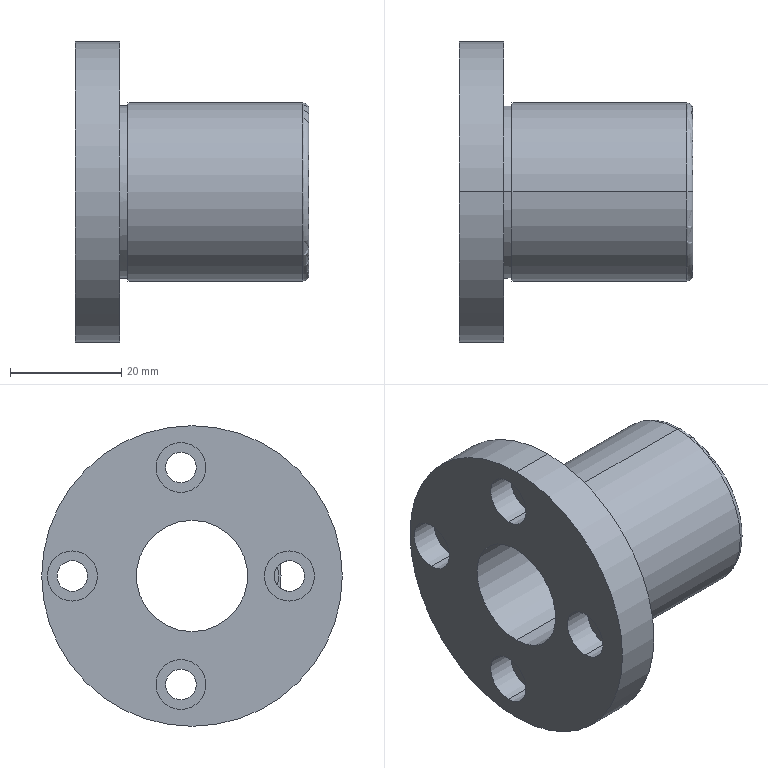Part | STEP file | LHFR20_LHTR20 | 1 solid | 35 faces | box 42 x 54 x 54 mm | volume 30800 mm3 | cylinder 24 | plane 9 | torus 2 | commonest cylinder face diameters 5.5 x8 9 x8 20 x2 31 x2 32 x2 54 x2
STEP:
#1=CARTESIAN_POINT('',(8.,-17.5,-2.75));
#2=VERTEX_POINT('',#1);
#3=CARTESIAN_POINT('',(8.,-17.5,2.75));
#4=VERTEX_POINT('',#3);
#5=CARTESIAN_POINT('',(8.,-17.5,0.));
#6=DIRECTION('',(-1.,0.,0.));
#7=DIRECTION('',(0.,0.,1.));
#8=AXIS2_PLACEMENT_3D('',#5,#6,#7);
#9=CIRCLE('',#8,2.75);
#10=EDGE_CURVE('',#2,#4,#9,.T.);
#11=ORIENTED_EDGE('',*,*,#10,.F.);
#12=CARTESIAN_POINT('',(5.1,-17.5,-2.75));
#13=VERTEX_POINT('',#12);
#14=CARTESIAN_POINT('',(8.,-17.5,-2.75));
#15=DIRECTION('',(-1.,0.,0.));
#16=VECTOR('',#15,1000.);
#17=LINE('',#14,#16);
#18=EDGE_CURVE('',#2,#13,#17,.T.);
#19=ORIENTED_EDGE('',*,*,#18,.T.);
#20=CARTESIAN_POINT('',(5.1,-17.5,2.75));
#21=VERTEX_POINT('',#20);
#22=CARTESIAN_POINT('',(5.1,-17.5,0.));
#23=DIRECTION('',(-1.,0.,0.));
#24=DIRECTION('',(0.,0.,1.));
#25=AXIS2_PLACEMENT_3D('',#22,#23,#24);
#26=CIRCLE('',#25,2.75);
#27=EDGE_CURVE('',#13,#21,#26,.T.);
#28=ORIENTED_EDGE('',*,*,#27,.T.);
#29=CARTESIAN_POINT('',(8.,-17.5,2.75));
#30=DIRECTION('',(-1.,0.,0.));
#31=VECTOR('',#30,1000.);
#32=LINE('',#29,#31);
#33=EDGE_CURVE('',#4,#21,#32,.T.);
#34=ORIENTED_EDGE('',*,*,#33,.F.);
#35=EDGE_LOOP('',(#11,#19,#28,#34));
#36=FACE_OUTER_BOUND('',#35,.T.);
#37=CARTESIAN_POINT('',(8.,-17.5,0.));
#38=DIRECTION('',(-1.,0.,0.));
#39=DIRECTION('',(0.,0.,1.));
#40=AXIS2_PLACEMENT_3D('',#37,#38,#39);
#41=CYLINDRICAL_SURFACE('',#40,2.75);
#42=ADVANCED_FACE('',(#36),#41,.F.);
#43=CARTESIAN_POINT('',(5.1,-17.5,-4.5));
#44=VERTEX_POINT('',#43);
#45=CARTESIAN_POINT('',(5.1,-17.5,4.5));
#46=VERTEX_POINT('',#45);
#47=CARTESIAN_POINT('',(5.1,-17.5,0.));
#48=DIRECTION('',(-1.,0.,0.));
#49=DIRECTION('',(0.,0.,1.));
#50=AXIS2_PLACEMENT_3D('',#47,#48,#49);
#51=CIRCLE('',#50,4.5);
#52=EDGE_CURVE('',#44,#46,#51,.T.);
#53=ORIENTED_EDGE('',*,*,#52,.F.);
#54=CARTESIAN_POINT('',(0.,-17.5,-4.5));
#55=VERTEX_POINT('',#54);
#56=CARTESIAN_POINT('',(8.,-17.5,-4.5));
#57=DIRECTION('',(-1.,0.,0.));
#58=VECTOR('',#57,1000.);
#59=LINE('',#56,#58);
#60=EDGE_CURVE('',#44,#55,#59,.T.);
#61=ORIENTED_EDGE('',*,*,#60,.T.);
#62=CARTESIAN_POINT('',(0.,-17.5,4.5));
#63=VERTEX_POINT('',#62);
#64=CARTESIAN_POINT('',(0.,-17.5,0.));
#65=DIRECTION('',(-1.,0.,0.));
#66=DIRECTION('',(0.,0.,1.));
#67=AXIS2_PLACEMENT_3D('',#64,#65,#66);
#68=CIRCLE('',#67,4.5);
#69=EDGE_CURVE('',#55,#63,#68,.T.);
#70=ORIENTED_EDGE('',*,*,#69,.T.);
#71=CARTESIAN_POINT('',(8.,-17.5,4.5));
#72=DIRECTION('',(-1.,0.,0.));
#73=VECTOR('',#72,1000.);
#74=LINE('',#71,#73);
#75=EDGE_CURVE('',#46,#63,#74,.T.);
#76=ORIENTED_EDGE('',*,*,#75,.F.);
#77=EDGE_LOOP('',(#53,#61,#70,#76));
#78=FACE_OUTER_BOUND('',#77,.T.);
#79=CARTESIAN_POINT('',(8.,-17.5,0.));
#80=DIRECTION('',(-1.,0.,0.));
#81=DIRECTION('',(0.,0.,1.));
#82=AXIS2_PLACEMENT_3D('',#79,#80,#81);
#83=CYLINDRICAL_SURFACE('',#82,4.5);
#84=ADVANCED_FACE('',(#78),#83,.F.);
#85=CARTESIAN_POINT('',(8.,2.,16.75));
#86=VERTEX_POINT('',#85);
#87=CARTESIAN_POINT('',(8.,2.,22.25));
#88=VERTEX_POINT('',#87);
#89=CARTESIAN_POINT('',(8.,2.,19.5));
#90=DIRECTION('',(-1.,0.,0.));
#91=DIRECTION('',(0.,0.,1.));
#92=AXIS2_PLACEMENT_3D('',#89,#90,#91);
#93=CIRCLE('',#92,2.75);
#94=EDGE_CURVE('',#86,#88,#93,.T.);
#95=ORIENTED_EDGE('',*,*,#94,.F.);
#96=CARTESIAN_POINT('',(5.1,2.,16.75));
#97=VERTEX_POINT('',#96);
#98=CARTESIAN_POINT('',(8.,2.,16.75));
#99=DIRECTION('',(-1.,0.,0.));
#100=VECTOR('',#99,1000.);
#101=LINE('',#98,#100);
#102=EDGE_CURVE('',#86,#97,#101,.T.);
#103=ORIENTED_EDGE('',*,*,#102,.T.);
#104=CARTESIAN_POINT('',(5.1,2.,22.25));
#105=VERTEX_POINT('',#104);
#106=CARTESIAN_POINT('',(5.1,2.,19.5));
#107=DIRECTION('',(-1.,0.,0.));
#108=DIRECTION('',(0.,0.,1.));
#109=AXIS2_PLACEMENT_3D('',#106,#107,#108);
#110=CIRCLE('',#109,2.75);
#111=EDGE_CURVE('',#97,#105,#110,.T.);
#112=ORIENTED_EDGE('',*,*,#111,.T.);
#113=CARTESIAN_POINT('',(8.,2.,22.25));
#114=DIRECTION('',(-1.,0.,0.));
#115=VECTOR('',#114,1000.);
#116=LINE('',#113,#115);
#117=EDGE_CURVE('',#88,#105,#116,.T.);
#118=ORIENTED_EDGE('',*,*,#117,.F.);
#119=EDGE_LOOP('',(#95,#103,#112,#118));
#120=FACE_OUTER_BOUND('',#119,.T.);
#121=CARTESIAN_POINT('',(8.,2.,19.5));
#122=DIRECTION('',(-1.,0.,0.));
#123=DIRECTION('',(0.,0.,1.));
#124=AXIS2_PLACEMENT_3D('',#121,#122,#123);
#125=CYLINDRICAL_SURFACE('',#124,2.75);
#126=ADVANCED_FACE('',(#120),#125,.F.);
#127=CARTESIAN_POINT('',(5.1,2.,15.));
#128=VERTEX_POINT('',#127);
#129=CARTESIAN_POINT('',(5.1,2.,24.));
#130=VERTEX_POINT('',#129);
#131=CARTESIAN_POINT('',(5.1,2.,19.5));
#132=DIRECTION('',(-1.,0.,0.));
#133=DIRECTION('',(0.,0.,1.));
#134=AXIS2_PLACEMENT_3D('',#131,#132,#133);
#135=CIRCLE('',#134,4.5);
#136=EDGE_CURVE('',#128,#130,#135,.T.);
#137=ORIENTED_EDGE('',*,*,#136,.F.);
#138=CARTESIAN_POINT('',(0.,2.,15.));
#139=VERTEX_POINT('',#138);
#140=CARTESIAN_POINT('',(8.,2.,15.));
#141=DIRECTION('',(-1.,0.,0.));
#142=VECTOR('',#141,1000.);
#143=LINE('',#140,#142);
#144=EDGE_CURVE('',#128,#139,#143,.T.);
#145=ORIENTED_EDGE('',*,*,#144,.T.);
#146=CARTESIAN_POINT('',(0.,2.,24.));
#147=VERTEX_POINT('',#146);
#148=CARTESIAN_POINT('',(0.,2.,19.5));
#149=DIRECTION('',(-1.,0.,0.));
#150=DIRECTION('',(0.,0.,1.));
#151=AXIS2_PLACEMENT_3D('',#148,#149,#150);
#152=CIRCLE('',#151,4.5);
#153=EDGE_CURVE('',#139,#147,#152,.T.);
#154=ORIENTED_EDGE('',*,*,#153,.T.);
#155=CARTESIAN_POINT('',(8.,2.,24.));
#156=DIRECTION('',(-1.,0.,0.));
#157=VECTOR('',#156,1000.);
#158=LINE('',#155,#157);
#159=EDGE_CURVE('',#130,#147,#158,.T.);
#160=ORIENTED_EDGE('',*,*,#159,.F.);
#161=EDGE_LOOP('',(#137,#145,#154,#160));
#162=FACE_OUTER_BOUND('',#161,.T.);
#163=CARTESIAN_POINT('',(8.,2.,19.5));
#164=DIRECTION('',(-1.,0.,0.));
#165=DIRECTION('',(0.,0.,1.));
#166=AXIS2_PLACEMENT_3D('',#163,#164,#165);
#167=CYLINDRICAL_SURFACE('',#166,4.5);
#168=ADVANCED_FACE('',(#162),#167,.F.);
#169=CARTESIAN_POINT('',(8.,2.,-22.25));
#170=VERTEX_POINT('',#169);
#171=CARTESIAN_POINT('',(8.,2.,-16.75));
#172=VERTEX_POINT('',#171);
#173=CARTESIAN_POINT('',(8.,2.,-19.5));
#174=DIRECTION('',(-1.,0.,0.));
#175=DIRECTION('',(0.,0.,1.));
#176=AXIS2_PLACEMENT_3D('',#173,#174,#175);
#177=CIRCLE('',#176,2.75);
#178=EDGE_CURVE('',#170,#172,#177,.T.);
#179=ORIENTED_EDGE('',*,*,#178,.F.);
#180=CARTESIAN_POINT('',(5.1,2.,-22.25));
#181=VERTEX_POINT('',#180);
#182=CARTESIAN_POINT('',(8.,2.,-22.25));
#183=DIRECTION('',(-1.,0.,0.));
#184=VECTOR('',#183,1000.);
#185=LINE('',#182,#184);
#186=EDGE_CURVE('',#170,#181,#185,.T.);
#187=ORIENTED_EDGE('',*,*,#186,.T.);
#188=CARTESIAN_POINT('',(5.1,2.,-16.75));
#189=VERTEX_POINT('',#188);
#190=CARTESIAN_POINT('',(5.1,2.,-19.5));
#191=DIRECTION('',(-1.,0.,0.));
#192=DIRECTION('',(0.,0.,1.));
#193=AXIS2_PLACEMENT_3D('',#190,#191,#192);
#194=CIRCLE('',#193,2.75);
#195=EDGE_CURVE('',#181,#189,#194,.T.);
#196=ORIENTED_EDGE('',*,*,#195,.T.);
#197=CARTESIAN_POINT('',(8.,2.,-16.75));
#198=DIRECTION('',(-1.,0.,0.));
#199=VECTOR('',#198,1000.);
#200=LINE('',#197,#199);
#201=EDGE_CURVE('',#172,#189,#200,.T.);
#202=ORIENTED_EDGE('',*,*,#201,.F.);
#203=EDGE_LOOP('',(#179,#187,#196,#202));
#204=FACE_OUTER_BOUND('',#203,.T.);
#205=CARTESIAN_POINT('',(8.,2.,-19.5));
#206=DIRECTION('',(-1.,0.,0.));
#207=DIRECTION('',(0.,0.,1.));
#208=AXIS2_PLACEMENT_3D('',#205,#206,#207);
#209=CYLINDRICAL_SURFACE('',#208,2.75);
#210=ADVANCED_FACE('',(#204),#209,.F.);
#211=CARTESIAN_POINT('',(5.1,2.,-24.));
#212=VERTEX_POINT('',#211);
#213=CARTESIAN_POINT('',(5.1,2.,-15.));
#214=VERTEX_POINT('',#213);
#215=CARTESIAN_POINT('',(5.1,2.,-19.5));
#216=DIRECTION('',(-1.,0.,0.));
#217=DIRECTION('',(0.,0.,1.));
#218=AXIS2_PLACEMENT_3D('',#215,#216,#217);
#219=CIRCLE('',#218,4.5);
#220=EDGE_CURVE('',#212,#214,#219,.T.);
#221=ORIENTED_EDGE('',*,*,#220,.F.);
#222=CARTESIAN_POINT('',(0.,2.,-24.));
#223=VERTEX_POINT('',#222);
#224=CARTESIAN_POINT('',(8.,2.,-24.));
#225=DIRECTION('',(-1.,0.,0.));
#226=VECTOR('',#225,1000.);
#227=LINE('',#224,#226);
#228=EDGE_CURVE('',#212,#223,#227,.T.);
#229=ORIENTED_EDGE('',*,*,#228,.T.);
#230=CARTESIAN_POINT('',(0.,2.,-15.));
#231=VERTEX_POINT('',#230);
#232=CARTESIAN_POINT('',(0.,2.,-19.5));
#233=DIRECTION('',(-1.,0.,0.));
#234=DIRECTION('',(0.,0.,1.));
#235=AXIS2_PLACEMENT_3D('',#232,#233,#234);
#236=CIRCLE('',#235,4.5);
#237=EDGE_CURVE('',#223,#231,#236,.T.);
#238=ORIENTED_EDGE('',*,*,#237,.T.);
#239=CARTESIAN_POINT('',(8.,2.,-15.));
#240=DIRECTION('',(-1.,0.,0.));
#241=VECTOR('',#240,1000.);
#242=LINE('',#239,#241);
#243=EDGE_CURVE('',#214,#231,#242,.T.);
#244=ORIENTED_EDGE('',*,*,#243,.F.);
#245=EDGE_LOOP('',(#221,#229,#238,#244));
#246=FACE_OUTER_BOUND('',#245,.T.);
#247=CARTESIAN_POINT('',(8.,2.,-19.5));
#248=DIRECTION('',(-1.,0.,0.));
#249=DIRECTION('',(0.,0.,1.));
#250=AXIS2_PLACEMENT_3D('',#247,#248,#249);
#251=CYLINDRICAL_SURFACE('',#250,4.5);
#252=ADVANCED_FACE('',(#246),#251,.F.);
#253=CARTESIAN_POINT('',(8.,21.5,-2.75));
#254=VERTEX_POINT('',#253);
#255=CARTESIAN_POINT('',(8.,21.5,2.75));
#256=VERTEX_POINT('',#255);
#257=CARTESIAN_POINT('',(8.,21.5,0.));
#258=DIRECTION('',(-1.,0.,0.));
#259=DIRECTION('',(0.,0.,1.));
#260=AXIS2_PLACEMENT_3D('',#257,#258,#259);
#261=CIRCLE('',#260,2.75);
#262=EDGE_CURVE('',#254,#256,#261,.T.);
#263=ORIENTED_EDGE('',*,*,#262,.F.);
#264=CARTESIAN_POINT('',(5.1,21.5,-2.75));
#265=VERTEX_POINT('',#264);
#266=CARTESIAN_POINT('',(8.,21.5,-2.75));
#267=DIRECTION('',(-1.,0.,0.));
#268=VECTOR('',#267,1000.);
#269=LINE('',#266,#268);
#270=EDGE_CURVE('',#254,#265,#269,.T.);
#271=ORIENTED_EDGE('',*,*,#270,.T.);
#272=CARTESIAN_POINT('',(5.1,21.5,2.75));
#273=VERTEX_POINT('',#272);
#274=CARTESIAN_POINT('',(5.1,21.5,0.));
#275=DIRECTION('',(-1.,0.,0.));
#276=DIRECTION('',(0.,0.,1.));
#277=AXIS2_PLACEMENT_3D('',#274,#275,#276);
#278=CIRCLE('',#277,2.75);
#279=EDGE_CURVE('',#265,#273,#278,.T.);
#280=ORIENTED_EDGE('',*,*,#279,.T.);
#281=CARTESIAN_POINT('',(8.,21.5,2.75));
#282=DIRECTION('',(-1.,0.,0.));
#283=VECTOR('',#282,1000.);
#284=LINE('',#281,#283);
#285=EDGE_CURVE('',#256,#273,#284,.T.);
#286=ORIENTED_EDGE('',*,*,#285,.F.);
#287=EDGE_LOOP('',(#263,#271,#280,#286));
#288=FACE_OUTER_BOUND('',#287,.T.);
#289=CARTESIAN_POINT('',(8.,21.5,0.));
#290=DIRECTION('',(-1.,0.,0.));
#291=DIRECTION('',(0.,0.,1.));
#292=AXIS2_PLACEMENT_3D('',#289,#290,#291);
#293=CYLINDRICAL_SURFACE('',#292,2.75);
#294=ADVANCED_FACE('',(#288),#293,.F.);
#295=CARTESIAN_POINT('',(5.1,21.5,-4.5));
#296=VERTEX_POINT('',#295);
#297=CARTESIAN_POINT('',(5.1,21.5,4.5));
#298=VERTEX_POINT('',#297);
#299=CARTESIAN_POINT('',(5.1,21.5,0.));
#300=DIRECTION('',(-1.,0.,0.));
#301=DIRECTION('',(0.,0.,1.));
#302=AXIS2_PLACEMENT_3D('',#299,#300,#301);
#303=CIRCLE('',#302,4.5);
#304=EDGE_CURVE('',#296,#298,#303,.T.);
#305=ORIENTED_EDGE('',*,*,#304,.F.);
#306=CARTESIAN_POINT('',(0.,21.5,-4.5));
#307=VERTEX_POINT('',#306);
#308=CARTESIAN_POINT('',(8.,21.5,-4.5));
#309=DIRECTION('',(-1.,0.,0.));
#310=VECTOR('',#309,1000.);
#311=LINE('',#308,#310);
#312=EDGE_CURVE('',#296,#307,#311,.T.);
#313=ORIENTED_EDGE('',*,*,#312,.T.);
#314=CARTESIAN_POINT('',(0.,21.5,4.5));
#315=VERTEX_POINT('',#314);
#316=CARTESIAN_POINT('',(0.,21.5,0.));
#317=DIRECTION('',(-1.,0.,0.));
#318=DIRECTION('',(0.,0.,1.));
#319=AXIS2_PLACEMENT_3D('',#316,#317,#318);
#320=CIRCLE('',#319,4.5);
#321=EDGE_CURVE('',#307,#315,#320,.T.);
#322=ORIENTED_EDGE('',*,*,#321,.T.);
#323=CARTESIAN_POINT('',(8.,21.5,4.5));
#324=DIRECTION('',(-1.,0.,0.));
#325=VECTOR('',#324,1000.);
#326=LINE('',#323,#325);
#327=EDGE_CURVE('',#298,#315,#326,.T.);
#328=ORIENTED_EDGE('',*,*,#327,.F.);
#329=EDGE_LOOP('',(#305,#313,#322,#328));
#330=FACE_OUTER_BOUND('',#329,.T.);
#331=CARTESIAN_POINT('',(8.,21.5,0.));
#332=DIRECTION('',(-1.,0.,0.));
#333=DIRECTION('',(0.,0.,1.));
#334=AXIS2_PLACEMENT_3D('',#331,#332,#333);
#335=CYLINDRICAL_SURFACE('',#334,4.5);
#336=ADVANCED_FACE('',(#330),#335,.F.);
#337=CARTESIAN_POINT('',(9.5,0.,15.5));
#338=VERTEX_POINT('',#337);
#339=CARTESIAN_POINT('',(9.5,0.,-15.5));
#340=VERTEX_POINT('',#339);
#341=CARTESIAN_POINT('',(9.5,0.,0.));
#342=DIRECTION('',(-1.,0.,0.));
#343=DIRECTION('',(0.,0.,1.));
#344=AXIS2_PLACEMENT_3D('',#341,#342,#343);
#345=CIRCLE('',#344,15.5);
#346=EDGE_CURVE('',#338,#340,#345,.T.);
#347=ORIENTED_EDGE('',*,*,#346,.T.);
#348=CARTESIAN_POINT('',(8.,0.,-15.5));
#349=VERTEX_POINT('',#348);
#350=CARTESIAN_POINT('',(42.,0.,-15.5));
#351=DIRECTION('',(-1.,0.,0.));
#352=VECTOR('',#351,1000.);
#353=LINE('',#350,#352);
#354=EDGE_CURVE('',#340,#349,#353,.T.);
#355=ORIENTED_EDGE('',*,*,#354,.T.);
#356=CARTESIAN_POINT('',(8.,0.,15.5));
#357=VERTEX_POINT('',#356);
#358=CARTESIAN_POINT('',(8.,0.,0.));
#359=DIRECTION('',(-1.,0.,0.));
#360=DIRECTION('',(0.,0.,1.));
#361=AXIS2_PLACEMENT_3D('',#358,#359,#360);
#362=CIRCLE('',#361,15.5);
#363=EDGE_CURVE('',#357,#349,#362,.T.);
#364=ORIENTED_EDGE('',*,*,#363,.F.);
#365=CARTESIAN_POINT('',(42.,0.,15.5));
#366=DIRECTION('',(-1.,0.,0.));
#367=VECTOR('',#366,1000.);
#368=LINE('',#365,#367);
#369=EDGE_CURVE('',#338,#357,#368,.T.);
#370=ORIENTED_EDGE('',*,*,#369,.F.);
#371=EDGE_LOOP('',(#347,#355,#364,#370));
#372=FACE_OUTER_BOUND('',#371,.T.);
#373=CARTESIAN_POINT('',(42.,0.,0.));
#374=DIRECTION('',(-1.,0.,0.));
#375=DIRECTION('',(0.,0.,1.));
#376=AXIS2_PLACEMENT_3D('',#373,#374,#375);
#377=CYLINDRICAL_SURFACE('',#376,15.5);
#378=ADVANCED_FACE('',(#372),#377,.T.);
#379=CARTESIAN_POINT('',(40.933,0.,16.));
#380=VERTEX_POINT('',#379);
#381=CARTESIAN_POINT('',(40.933,0.,-16.));
#382=VERTEX_POINT('',#381);
#383=CARTESIAN_POINT('',(40.933,0.,0.));
#384=DIRECTION('',(-1.,0.,0.));
#385=DIRECTION('',(0.,0.,1.));
#386=AXIS2_PLACEMENT_3D('',#383,#384,#385);
#387=CIRCLE('',#386,16.);
#388=EDGE_CURVE('',#380,#382,#387,.T.);
#389=ORIENTED_EDGE('',*,*,#388,.T.);
#390=CARTESIAN_POINT('',(9.5,0.,-16.));
#391=VERTEX_POINT('',#390);
#392=CARTESIAN_POINT('',(42.,0.,-16.));
#393=DIRECTION('',(-1.,0.,0.));
#394=VECTOR('',#393,1000.);
#395=LINE('',#392,#394);
#396=EDGE_CURVE('',#382,#391,#395,.T.);
#397=ORIENTED_EDGE('',*,*,#396,.T.);
#398=CARTESIAN_POINT('',(9.5,0.,16.));
#399=VERTEX_POINT('',#398);
#400=CARTESIAN_POINT('',(9.5,0.,0.));
#401=DIRECTION('',(-1.,0.,0.));
#402=DIRECTION('',(0.,0.,1.));
#403=AXIS2_PLACEMENT_3D('',#400,#401,#402);
#404=CIRCLE('',#403,16.);
#405=EDGE_CURVE('',#399,#391,#404,.T.);
#406=ORIENTED_EDGE('',*,*,#405,.F.);
#407=CARTESIAN_POINT('',(42.,0.,16.));
#408=DIRECTION('',(-1.,0.,0.));
#409=VECTOR('',#408,1000.);
#410=LINE('',#407,#409);
#411=EDGE_CURVE('',#380,#399,#410,.T.);
#412=ORIENTED_EDGE('',*,*,#411,.F.);
#413=EDGE_LOOP('',(#389,#397,#406,#412));
#414=FACE_OUTER_BOUND('',#413,.T.);
#415=CARTESIAN_POINT('',(42.,0.,0.));
#416=DIRECTION('',(-1.,0.,0.));
#417=DIRECTION('',(0.,0.,1.));
#418=AXIS2_PLACEMENT_3D('',#415,#416,#417);
#419=CYLINDRICAL_SURFACE('',#418,16.);
#420=ADVANCED_FACE('',(#414),#419,.T.);
#421=CARTESIAN_POINT('',(42.,0.,14.933));
#422=VERTEX_POINT('',#421);
#423=CARTESIAN_POINT('',(42.,0.,-14.933));
#424=VERTEX_POINT('',#423);
#425=CARTESIAN_POINT('',(42.,0.,0.));
#426=DIRECTION('',(-1.,0.,0.));
#427=DIRECTION('',(0.,0.,1.));
#428=AXIS2_PLACEMENT_3D('',#425,#426,#427);
#429=CIRCLE('',#428,14.933);
#430=EDGE_CURVE('',#422,#424,#429,.T.);
#431=ORIENTED_EDGE('',*,*,#430,.T.);
#432=CARTESIAN_POINT('',(40.933,0.,-14.933));
#433=DIRECTION('',(0.,1.,0.));
#434=DIRECTION('',(0.,0.,1.));
#435=AXIS2_PLACEMENT_3D('',#432,#433,#434);
#436=CIRCLE('',#435,1.067);
#437=EDGE_CURVE('',#424,#382,#436,.T.);
#438=ORIENTED_EDGE('',*,*,#437,.T.);
#439=ORIENTED_EDGE('',*,*,#388,.F.);
#440=CARTESIAN_POINT('',(40.933,0.,14.933));
#441=DIRECTION('',(0.,-1.,0.));
#442=DIRECTION('',(0.,0.,-1.));
#443=AXIS2_PLACEMENT_3D('',#440,#441,#442);
#444=CIRCLE('',#443,1.067);
#445=EDGE_CURVE('',#422,#380,#444,.T.);
#446=ORIENTED_EDGE('',*,*,#445,.F.);
#447=EDGE_LOOP('',(#431,#438,#439,#446));
#448=FACE_OUTER_BOUND('',#447,.T.);
#449=CARTESIAN_POINT('',(40.933,0.,0.));
#450=DIRECTION('',(-1.,0.,0.));
#451=DIRECTION('',(0.,0.,1.));
#452=AXIS2_PLACEMENT_3D('',#449,#450,#451);
#453=TOROIDAL_SURFACE('',#452,14.933,1.067);
#454=ADVANCED_FACE('',(#448),#453,.T.);
#455=CARTESIAN_POINT('',(42.,0.,-10.));
#456=VERTEX_POINT('',#455);
#457=CARTESIAN_POINT('',(42.,0.,10.));
#458=VERTEX_POINT('',#457);
#459=CARTESIAN_POINT('',(42.,0.,0.));
#460=DIRECTION('',(-1.,0.,0.));
#461=DIRECTION('',(0.,0.,1.));
#462=AXIS2_PLACEMENT_3D('',#459,#460,#461);
#463=CIRCLE('',#462,10.);
#464=EDGE_CURVE('',#456,#458,#463,.T.);
#465=ORIENTED_EDGE('',*,*,#464,.F.);
#466=CARTESIAN_POINT('',(0.,0.,-10.));
#467=VERTEX_POINT('',#466);
#468=CARTESIAN_POINT('',(42.,0.,-10.));
#469=DIRECTION('',(-1.,0.,0.));
#470=VECTOR('',#469,1000.);
#471=LINE('',#468,#470);
#472=EDGE_CURVE('',#456,#467,#471,.T.);
#473=ORIENTED_EDGE('',*,*,#472,.T.);
#474=CARTESIAN_POINT('',(0.,0.,10.));
#475=VERTEX_POINT('',#474);
#476=CARTESIAN_POINT('',(0.,0.,0.));
#477=DIRECTION('',(-1.,0.,0.));
#478=DIRECTION('',(0.,0.,1.));
#479=AXIS2_PLACEMENT_3D('',#476,#477,#478);
#480=CIRCLE('',#479,10.);
#481=EDGE_CURVE('',#467,#475,#480,.T.);
#482=ORIENTED_EDGE('',*,*,#481,.T.);
#483=CARTESIAN_POINT('',(42.,0.,10.));
#484=DIRECTION('',(-1.,0.,0.));
#485=VECTOR('',#484,1000.);
#486=LINE('',#483,#485);
#487=EDGE_CURVE('',#458,#475,#486,.T.);
#488=ORIENTED_EDGE('',*,*,#487,.F.);
#489=EDGE_LOOP('',(#465,#473,#482,#488));
#490=FACE_OUTER_BOUND('',#489,.T.);
#491=CARTESIAN_POINT('',(42.,0.,0.));
#492=DIRECTION('',(-1.,0.,0.));
#493=DIRECTION('',(0.,0.,1.));
#494=AXIS2_PLACEMENT_3D('',#491,#492,#493);
#495=CYLINDRICAL_SURFACE('',#494,10.);
#496=ADVANCED_FACE('',(#490),#495,.F.);
#497=CARTESIAN_POINT('',(8.,0.,27.));
#498=VERTEX_POINT('',#497);
#499=CARTESIAN_POINT('',(8.,0.,-27.));
#500=VERTEX_POINT('',#499);
#501=CARTESIAN_POINT('',(8.,0.,0.));
#502=DIRECTION('',(-1.,0.,0.));
#503=DIRECTION('',(0.,0.,1.));
#504=AXIS2_PLACEMENT_3D('',#501,#502,#503);
#505=CIRCLE('',#504,27.);
#506=EDGE_CURVE('',#498,#500,#505,.T.);
#507=ORIENTED_EDGE('',*,*,#506,.T.);
#508=CARTESIAN_POINT('',(0.,0.,-27.));
#509=VERTEX_POINT('',#508);
#510=CARTESIAN_POINT('',(42.,0.,-27.));
#511=DIRECTION('',(-1.,0.,0.));
#512=VECTOR('',#511,1000.);
#513=LINE('',#510,#512);
#514=EDGE_CURVE('',#500,#509,#513,.T.);
#515=ORIENTED_EDGE('',*,*,#514,.T.);
#516=CARTESIAN_POINT('',(0.,0.,27.));
#517=VERTEX_POINT('',#516);
#518=CARTESIAN_POINT('',(0.,0.,0.));
#519=DIRECTION('',(-1.,0.,0.));
#520=DIRECTION('',(0.,0.,1.));
#521=AXIS2_PLACEMENT_3D('',#518,#519,#520);
#522=CIRCLE('',#521,27.);
#523=EDGE_CURVE('',#517,#509,#522,.T.);
#524=ORIENTED_EDGE('',*,*,#523,.F.);
#525=CARTESIAN_POINT('',(42.,0.,27.));
#526=DIRECTION('',(-1.,0.,0.));
#527=VECTOR('',#526,1000.);
#528=LINE('',#525,#527);
#529=EDGE_CURVE('',#498,#517,#528,.T.);
#530=ORIENTED_EDGE('',*,*,#529,.F.);
#531=EDGE_LOOP('',(#507,#515,#524,#530));
#532=FACE_OUTER_BOUND('',#531,.T.);
#533=CARTESIAN_POINT('',(42.,0.,0.));
#534=DIRECTION('',(-1.,0.,0.));
#535=DIRECTION('',(0.,0.,1.));
#536=AXIS2_PLACEMENT_3D('',#533,#534,#535);
#537=CYLINDRICAL_SURFACE('',#536,27.);
#538=ADVANCED_FACE('',(#532),#537,.T.);
#539=CARTESIAN_POINT('',(0.,2.,19.5));
#540=DIRECTION('',(-1.,0.,0.));
#541=DIRECTION('',(0.,0.,1.));
#542=AXIS2_PLACEMENT_3D('',#539,#540,#541);
#543=CIRCLE('',#542,4.5);
#544=EDGE_CURVE('',#147,#139,#543,.T.);
#545=ORIENTED_EDGE('',*,*,#544,.F.);
#546=ORIENTED_EDGE('',*,*,#153,.F.);
#547=EDGE_LOOP('',(#545,#546));
#548=FACE_BOUND('',#547,.T.);
#549=CARTESIAN_POINT('',(0.,21.5,0.));
#550=DIRECTION('',(-1.,0.,0.));
#551=DIRECTION('',(0.,0.,1.));
#552=AXIS2_PLACEMENT_3D('',#549,#550,#551);
#553=CIRCLE('',#552,4.5);
#554=EDGE_CURVE('',#315,#307,#553,.T.);
#555=ORIENTED_EDGE('',*,*,#554,.F.);
#556=ORIENTED_EDGE('',*,*,#321,.F.);
#557=EDGE_LOOP('',(#555,#556));
#558=FACE_BOUND('',#557,.T.);
#559=CARTESIAN_POINT('',(0.,0.,0.));
#560=DIRECTION('',(-1.,0.,0.));
#561=DIRECTION('',(0.,0.,1.));
#562=AXIS2_PLACEMENT_3D('',#559,#560,#561);
#563=CIRCLE('',#562,10.);
#564=EDGE_CURVE('',#475,#467,#563,.T.);
#565=ORIENTED_EDGE('',*,*,#564,.F.);
#566=ORIENTED_EDGE('',*,*,#481,.F.);
#567=EDGE_LOOP('',(#565,#566));
#568=FACE_BOUND('',#567,.T.);
#569=ORIENTED_EDGE('',*,*,#523,.T.);
#570=CARTESIAN_POINT('',(0.,0.,0.));
#571=DIRECTION('',(-1.,0.,0.));
#572=DIRECTION('',(0.,0.,1.));
#573=AXIS2_PLACEMENT_3D('',#570,#571,#572);
#574=CIRCLE('',#573,27.);
#575=EDGE_CURVE('',#509,#517,#574,.T.);
#576=ORIENTED_EDGE('',*,*,#575,.T.);
#577=EDGE_LOOP('',(#569,#576));
#578=FACE_OUTER_BOUND('',#577,.T.);
#579=CARTESIAN_POINT('',(0.,2.,-19.5));
#580=DIRECTION('',(-1.,0.,0.));
#581=DIRECTION('',(0.,0.,1.));
#582=AXIS2_PLACEMENT_3D('',#579,#580,#581);
#583=CIRCLE('',#582,4.5);
#584=EDGE_CURVE('',#231,#223,#583,.T.);
#585=ORIENTED_EDGE('',*,*,#584,.F.);
#586=ORIENTED_EDGE('',*,*,#237,.F.);
#587=EDGE_LOOP('',(#585,#586));
#588=FACE_BOUND('',#587,.T.);
#589=CARTESIAN_POINT('',(0.,-17.5,0.));
#590=DIRECTION('',(-1.,0.,0.));
#591=DIRECTION('',(0.,0.,1.));
#592=AXIS2_PLACEMENT_3D('',#589,#590,#591);
#593=CIRCLE('',#592,4.5);
#594=EDGE_CURVE('',#63,#55,#593,.T.);
#595=ORIENTED_EDGE('',*,*,#594,.F.);
#596=ORIENTED_EDGE('',*,*,#69,.F.);
#597=EDGE_LOOP('',(#595,#596));
#598=FACE_BOUND('',#597,.T.);
#599=CARTESIAN_POINT('',(0.,27.,0.));
#600=DIRECTION('',(1.,0.,0.));
#601=DIRECTION('',(0.,0.,-1.));
#602=AXIS2_PLACEMENT_3D('',#599,#600,#601);
#603=PLANE('',#602);
#604=ADVANCED_FACE('',(#548,#558,#568,#578,#588,#598),#603,.F.);
#605=CARTESIAN_POINT('',(8.,2.,19.5));
#606=DIRECTION('',(-1.,0.,0.));
#607=DIRECTION('',(0.,0.,1.));
#608=AXIS2_PLACEMENT_3D('',#605,#606,#607);
#609=CIRCLE('',#608,2.75);
#610=EDGE_CURVE('',#88,#86,#609,.T.);
#611=ORIENTED_EDGE('',*,*,#610,.T.);
#612=ORIENTED_EDGE('',*,*,#94,.T.);
#613=EDGE_LOOP('',(#611,#612));
#614=FACE_BOUND('',#613,.T.);
#615=CARTESIAN_POINT('',(8.,21.5,0.));
#616=DIRECTION('',(-1.,0.,0.));
#617=DIRECTION('',(0.,0.,1.));
#618=AXIS2_PLACEMENT_3D('',#615,#616,#617);
#619=CIRCLE('',#618,2.75);
#620=EDGE_CURVE('',#256,#254,#619,.T.);
#621=ORIENTED_EDGE('',*,*,#620,.T.);
#622=ORIENTED_EDGE('',*,*,#262,.T.);
#623=EDGE_LOOP('',(#621,#622));
#624=FACE_BOUND('',#623,.T.);
#625=ORIENTED_EDGE('',*,*,#506,.F.);
#626=CARTESIAN_POINT('',(8.,0.,0.));
#627=DIRECTION('',(-1.,0.,0.));
#628=DIRECTION('',(0.,0.,1.));
#629=AXIS2_PLACEMENT_3D('',#626,#627,#628);
#630=CIRCLE('',#629,27.);
#631=EDGE_CURVE('',#500,#498,#630,.T.);
#632=ORIENTED_EDGE('',*,*,#631,.F.);
#633=EDGE_LOOP('',(#625,#632));
#634=FACE_OUTER_BOUND('',#633,.T.);
#635=CARTESIAN_POINT('',(8.,2.,-19.5));
#636=DIRECTION('',(-1.,0.,0.));
#637=DIRECTION('',(0.,0.,1.));
#638=AXIS2_PLACEMENT_3D('',#635,#636,#637);
#639=CIRCLE('',#638,2.75);
#640=EDGE_CURVE('',#172,#170,#639,.T.);
#641=ORIENTED_EDGE('',*,*,#640,.T.);
#642=ORIENTED_EDGE('',*,*,#178,.T.);
#643=EDGE_LOOP('',(#641,#642));
#644=FACE_BOUND('',#643,.T.);
#645=CARTESIAN_POINT('',(8.,-15.398,-1.773));
#646=VERTEX_POINT('',#645);
#647=CARTESIAN_POINT('',(8.,-17.5,0.));
#648=DIRECTION('',(-1.,0.,0.));
#649=DIRECTION('',(0.,0.,1.));
#650=AXIS2_PLACEMENT_3D('',#647,#648,#649);
#651=CIRCLE('',#650,2.75);
#652=EDGE_CURVE('',#646,#2,#651,.T.);
#653=ORIENTED_EDGE('',*,*,#652,.T.);
#654=ORIENTED_EDGE('',*,*,#10,.T.);
#655=CARTESIAN_POINT('',(8.,-15.398,1.773));
#656=VERTEX_POINT('',#655);
#657=CARTESIAN_POINT('',(8.,-17.5,0.));
#658=DIRECTION('',(-1.,0.,0.));
#659=DIRECTION('',(0.,0.,1.));
#660=AXIS2_PLACEMENT_3D('',#657,#658,#659);
#661=CIRCLE('',#660,2.75);
#662=EDGE_CURVE('',#4,#656,#661,.T.);
#663=ORIENTED_EDGE('',*,*,#662,.T.);
#664=CARTESIAN_POINT('',(8.,0.,0.));
#665=DIRECTION('',(-1.,0.,0.));
#666=DIRECTION('',(0.,0.,1.));
#667=AXIS2_PLACEMENT_3D('',#664,#665,#666);
#668=CIRCLE('',#667,15.5);
#669=EDGE_CURVE('',#656,#357,#668,.T.);
#670=ORIENTED_EDGE('',*,*,#669,.T.);
#671=ORIENTED_EDGE('',*,*,#363,.T.);
#672=CARTESIAN_POINT('',(8.,0.,0.));
#673=DIRECTION('',(-1.,0.,0.));
#674=DIRECTION('',(0.,0.,1.));
#675=AXIS2_PLACEMENT_3D('',#672,#673,#674);
#676=CIRCLE('',#675,15.5);
#677=EDGE_CURVE('',#349,#646,#676,.T.);
#678=ORIENTED_EDGE('',*,*,#677,.T.);
#679=EDGE_LOOP('',(#653,#654,#663,#670,#671,#678));
#680=FACE_BOUND('',#679,.T.);
#681=CARTESIAN_POINT('',(8.,15.5,0.));
#682=DIRECTION('',(-1.,0.,0.));
#683=DIRECTION('',(0.,0.,1.));
#684=AXIS2_PLACEMENT_3D('',#681,#682,#683);
#685=PLANE('',#684);
#686=ADVANCED_FACE('',(#614,#624,#634,#644,#680),#685,.F.);
#687=ORIENTED_EDGE('',*,*,#514,.F.);
#688=ORIENTED_EDGE('',*,*,#631,.T.);
#689=ORIENTED_EDGE('',*,*,#529,.T.);
#690=ORIENTED_EDGE('',*,*,#575,.F.);
#691=EDGE_LOOP('',(#687,#688,#689,#690));
#692=FACE_OUTER_BOUND('',#691,.T.);
#693=CARTESIAN_POINT('',(42.,0.,0.));
#694=DIRECTION('',(-1.,0.,0.));
#695=DIRECTION('',(0.,0.,1.));
#696=AXIS2_PLACEMENT_3D('',#693,#694,#695);
#697=CYLINDRICAL_SURFACE('',#696,27.);
#698=ADVANCED_FACE('',(#692),#697,.T.);
#699=ORIENTED_EDGE('',*,*,#472,.F.);
#700=CARTESIAN_POINT('',(42.,0.,0.));
#701=DIRECTION('',(-1.,0.,0.));
#702=DIRECTION('',(0.,0.,1.));
#703=AXIS2_PLACEMENT_3D('',#700,#701,#702);
#704=CIRCLE('',#703,10.);
#705=EDGE_CURVE('',#458,#456,#704,.T.);
#706=ORIENTED_EDGE('',*,*,#705,.F.);
#707=ORIENTED_EDGE('',*,*,#487,.T.);
#708=ORIENTED_EDGE('',*,*,#564,.T.);
#709=EDGE_LOOP('',(#699,#706,#707,#708));
#710=FACE_OUTER_BOUND('',#709,.T.);
#711=CARTESIAN_POINT('',(42.,0.,0.));
#712=DIRECTION('',(-1.,0.,0.));
#713=DIRECTION('',(0.,0.,1.));
#714=AXIS2_PLACEMENT_3D('',#711,#712,#713);
#715=CYLINDRICAL_SURFACE('',#714,10.);
#716=ADVANCED_FACE('',(#710),#715,.F.);
#717=ORIENTED_EDGE('',*,*,#430,.F.);
#718=CARTESIAN_POINT('',(42.,0.,0.));
#719=DIRECTION('',(-1.,0.,0.));
#720=DIRECTION('',(0.,0.,1.));
#721=AXIS2_PLACEMENT_3D('',#718,#719,#720);
#722=CIRCLE('',#721,14.933);
#723=EDGE_CURVE('',#424,#422,#722,.T.);
#724=ORIENTED_EDGE('',*,*,#723,.F.);
#725=EDGE_LOOP('',(#717,#724));
#726=FACE_OUTER_BOUND('',#725,.T.);
#727=ORIENTED_EDGE('',*,*,#705,.T.);
#728=ORIENTED_EDGE('',*,*,#464,.T.);
#729=EDGE_LOOP('',(#727,#728));
#730=FACE_BOUND('',#729,.T.);
#731=CARTESIAN_POINT('',(42.,10.,0.));
#732=DIRECTION('',(-1.,0.,0.));
#733=DIRECTION('',(0.,0.,1.));
#734=AXIS2_PLACEMENT_3D('',#731,#732,#733);
#735=PLANE('',#734);
#736=ADVANCED_FACE('',(#726,#730),#735,.F.);
#737=ORIENTED_EDGE('',*,*,#437,.F.);
#738=ORIENTED_EDGE('',*,*,#723,.T.);
#739=ORIENTED_EDGE('',*,*,#445,.T.);
#740=CARTESIAN_POINT('',(40.933,0.,0.));
#741=DIRECTION('',(-1.,0.,0.));
#742=DIRECTION('',(0.,0.,1.));
#743=AXIS2_PLACEMENT_3D('',#740,#741,#742);
#744=CIRCLE('',#743,16.);
#745=EDGE_CURVE('',#382,#380,#744,.T.);
#746=ORIENTED_EDGE('',*,*,#745,.F.);
#747=EDGE_LOOP('',(#737,#738,#739,#746));
#748=FACE_OUTER_BOUND('',#747,.T.);
#749=CARTESIAN_POINT('',(40.933,0.,0.));
#750=DIRECTION('',(-1.,0.,0.));
#751=DIRECTION('',(0.,0.,1.));
#752=AXIS2_PLACEMENT_3D('',#749,#750,#751);
#753=TOROIDAL_SURFACE('',#752,14.933,1.067);
#754=ADVANCED_FACE('',(#748),#753,.T.);
#755=ORIENTED_EDGE('',*,*,#396,.F.);
#756=ORIENTED_EDGE('',*,*,#745,.T.);
#757=ORIENTED_EDGE('',*,*,#411,.T.);
#758=CARTESIAN_POINT('',(9.5,0.,0.));
#759=DIRECTION('',(-1.,0.,0.));
#760=DIRECTION('',(0.,0.,1.));
#761=AXIS2_PLACEMENT_3D('',#758,#759,#760);
#762=CIRCLE('',#761,16.);
#763=EDGE_CURVE('',#391,#399,#762,.T.);
#764=ORIENTED_EDGE('',*,*,#763,.F.);
#765=EDGE_LOOP('',(#755,#756,#757,#764));
#766=FACE_OUTER_BOUND('',#765,.T.);
#767=CARTESIAN_POINT('',(42.,0.,0.));
#768=DIRECTION('',(-1.,0.,0.));
#769=DIRECTION('',(0.,0.,1.));
#770=AXIS2_PLACEMENT_3D('',#767,#768,#769);
#771=CYLINDRICAL_SURFACE('',#770,16.);
#772=ADVANCED_FACE('',(#766),#771,.T.);
#773=ORIENTED_EDGE('',*,*,#346,.F.);
#774=CARTESIAN_POINT('',(9.5,0.,0.));
#775=DIRECTION('',(-1.,0.,0.));
#776=DIRECTION('',(0.,0.,1.));
#777=AXIS2_PLACEMENT_3D('',#774,#775,#776);
#778=CIRCLE('',#777,15.5);
#779=EDGE_CURVE('',#340,#338,#778,.T.);
#780=ORIENTED_EDGE('',*,*,#779,.F.);
#781=EDGE_LOOP('',(#773,#780));
#782=FACE_BOUND('',#781,.T.);
#783=ORIENTED_EDGE('',*,*,#405,.T.);
#784=ORIENTED_EDGE('',*,*,#763,.T.);
#785=EDGE_LOOP('',(#783,#784));
#786=FACE_OUTER_BOUND('',#785,.T.);
#787=CARTESIAN_POINT('',(9.5,16.,0.));
#788=DIRECTION('',(1.,0.,0.));
#789=DIRECTION('',(0.,0.,-1.));
#790=AXIS2_PLACEMENT_3D('',#787,#788,#789);
#791=PLANE('',#790);
#792=ADVANCED_FACE('',(#782,#786),#791,.F.);
#793=ORIENTED_EDGE('',*,*,#354,.F.);
#794=ORIENTED_EDGE('',*,*,#779,.T.);
#795=ORIENTED_EDGE('',*,*,#369,.T.);
#796=ORIENTED_EDGE('',*,*,#669,.F.);
#797=CARTESIAN_POINT('',(8.,0.,0.));
#798=DIRECTION('',(-1.,0.,0.));
#799=DIRECTION('',(0.,0.,1.));
#800=AXIS2_PLACEMENT_3D('',#797,#798,#799);
#801=CIRCLE('',#800,15.5);
#802=EDGE_CURVE('',#646,#656,#801,.T.);
#803=ORIENTED_EDGE('',*,*,#802,.F.);
#804=ORIENTED_EDGE('',*,*,#677,.F.);
#805=EDGE_LOOP('',(#793,#794,#795,#796,#803,#804));
#806=FACE_OUTER_BOUND('',#805,.T.);
#807=CARTESIAN_POINT('',(42.,0.,0.));
#808=DIRECTION('',(-1.,0.,0.));
#809=DIRECTION('',(0.,0.,1.));
#810=AXIS2_PLACEMENT_3D('',#807,#808,#809);
#811=CYLINDRICAL_SURFACE('',#810,15.5);
#812=ADVANCED_FACE('',(#806),#811,.T.);
#813=ORIENTED_EDGE('',*,*,#312,.F.);
#814=CARTESIAN_POINT('',(5.1,21.5,0.));
#815=DIRECTION('',(-1.,0.,0.));
#816=DIRECTION('',(0.,0.,1.));
#817=AXIS2_PLACEMENT_3D('',#814,#815,#816);
#818=CIRCLE('',#817,4.5);
#819=EDGE_CURVE('',#298,#296,#818,.T.);
#820=ORIENTED_EDGE('',*,*,#819,.F.);
#821=ORIENTED_EDGE('',*,*,#327,.T.);
#822=ORIENTED_EDGE('',*,*,#554,.T.);
#823=EDGE_LOOP('',(#813,#820,#821,#822));
#824=FACE_OUTER_BOUND('',#823,.T.);
#825=CARTESIAN_POINT('',(8.,21.5,0.));
#826=DIRECTION('',(-1.,0.,0.));
#827=DIRECTION('',(0.,0.,1.));
#828=AXIS2_PLACEMENT_3D('',#825,#826,#827);
#829=CYLINDRICAL_SURFACE('',#828,4.5);
#830=ADVANCED_FACE('',(#824),#829,.F.);
#831=ORIENTED_EDGE('',*,*,#819,.T.);
#832=ORIENTED_EDGE('',*,*,#304,.T.);
#833=EDGE_LOOP('',(#831,#832));
#834=FACE_OUTER_BOUND('',#833,.T.);
#835=CARTESIAN_POINT('',(5.1,21.5,0.));
#836=DIRECTION('',(-1.,0.,0.));
#837=DIRECTION('',(0.,0.,1.));
#838=AXIS2_PLACEMENT_3D('',#835,#836,#837);
#839=CIRCLE('',#838,2.75);
#840=EDGE_CURVE('',#273,#265,#839,.T.);
#841=ORIENTED_EDGE('',*,*,#840,.F.);
#842=ORIENTED_EDGE('',*,*,#279,.F.);
#843=EDGE_LOOP('',(#841,#842));
#844=FACE_BOUND('',#843,.T.);
#845=CARTESIAN_POINT('',(5.1,24.25,0.));
#846=DIRECTION('',(-1.,0.,0.));
#847=DIRECTION('',(0.,0.,1.));
#848=AXIS2_PLACEMENT_3D('',#845,#846,#847);
#849=PLANE('',#848);
#850=ADVANCED_FACE('',(#834,#844),#849,.T.);
#851=ORIENTED_EDGE('',*,*,#270,.F.);
#852=ORIENTED_EDGE('',*,*,#620,.F.);
#853=ORIENTED_EDGE('',*,*,#285,.T.);
#854=ORIENTED_EDGE('',*,*,#840,.T.);
#855=EDGE_LOOP('',(#851,#852,#853,#854));
#856=FACE_OUTER_BOUND('',#855,.T.);
#857=CARTESIAN_POINT('',(8.,21.5,0.));
#858=DIRECTION('',(-1.,0.,0.));
#859=DIRECTION('',(0.,0.,1.));
#860=AXIS2_PLACEMENT_3D('',#857,#858,#859);
#861=CYLINDRICAL_SURFACE('',#860,2.75);
#862=ADVANCED_FACE('',(#856),#861,.F.);
#863=ORIENTED_EDGE('',*,*,#228,.F.);
#864=CARTESIAN_POINT('',(5.1,2.,-19.5));
#865=DIRECTION('',(-1.,0.,0.));
#866=DIRECTION('',(0.,0.,1.));
#867=AXIS2_PLACEMENT_3D('',#864,#865,#866);
#868=CIRCLE('',#867,4.5);
#869=EDGE_CURVE('',#214,#212,#868,.T.);
#870=ORIENTED_EDGE('',*,*,#869,.F.);
#871=ORIENTED_EDGE('',*,*,#243,.T.);
#872=ORIENTED_EDGE('',*,*,#584,.T.);
#873=EDGE_LOOP('',(#863,#870,#871,#872));
#874=FACE_OUTER_BOUND('',#873,.T.);
#875=CARTESIAN_POINT('',(8.,2.,-19.5));
#876=DIRECTION('',(-1.,0.,0.));
#877=DIRECTION('',(0.,0.,1.));
#878=AXIS2_PLACEMENT_3D('',#875,#876,#877);
#879=CYLINDRICAL_SURFACE('',#878,4.5);
#880=ADVANCED_FACE('',(#874),#879,.F.);
#881=ORIENTED_EDGE('',*,*,#869,.T.);
#882=ORIENTED_EDGE('',*,*,#220,.T.);
#883=EDGE_LOOP('',(#881,#882));
#884=FACE_OUTER_BOUND('',#883,.T.);
#885=CARTESIAN_POINT('',(5.1,2.,-19.5));
#886=DIRECTION('',(-1.,0.,0.));
#887=DIRECTION('',(0.,0.,1.));
#888=AXIS2_PLACEMENT_3D('',#885,#886,#887);
#889=CIRCLE('',#888,2.75);
#890=EDGE_CURVE('',#189,#181,#889,.T.);
#891=ORIENTED_EDGE('',*,*,#890,.F.);
#892=ORIENTED_EDGE('',*,*,#195,.F.);
#893=EDGE_LOOP('',(#891,#892));
#894=FACE_BOUND('',#893,.T.);
#895=CARTESIAN_POINT('',(5.1,4.75,-19.5));
#896=DIRECTION('',(-1.,0.,0.));
#897=DIRECTION('',(0.,0.,1.));
#898=AXIS2_PLACEMENT_3D('',#895,#896,#897);
#899=PLANE('',#898);
#900=ADVANCED_FACE('',(#884,#894),#899,.T.);
#901=ORIENTED_EDGE('',*,*,#186,.F.);
#902=ORIENTED_EDGE('',*,*,#640,.F.);
#903=ORIENTED_EDGE('',*,*,#201,.T.);
#904=ORIENTED_EDGE('',*,*,#890,.T.);
#905=EDGE_LOOP('',(#901,#902,#903,#904));
#906=FACE_OUTER_BOUND('',#905,.T.);
#907=CARTESIAN_POINT('',(8.,2.,-19.5));
#908=DIRECTION('',(-1.,0.,0.));
#909=DIRECTION('',(0.,0.,1.));
#910=AXIS2_PLACEMENT_3D('',#907,#908,#909);
#911=CYLINDRICAL_SURFACE('',#910,2.75);
#912=ADVANCED_FACE('',(#906),#911,.F.);
#913=ORIENTED_EDGE('',*,*,#144,.F.);
#914=CARTESIAN_POINT('',(5.1,2.,19.5));
#915=DIRECTION('',(-1.,0.,0.));
#916=DIRECTION('',(0.,0.,1.));
#917=AXIS2_PLACEMENT_3D('',#914,#915,#916);
#918=CIRCLE('',#917,4.5);
#919=EDGE_CURVE('',#130,#128,#918,.T.);
#920=ORIENTED_EDGE('',*,*,#919,.F.);
#921=ORIENTED_EDGE('',*,*,#159,.T.);
#922=ORIENTED_EDGE('',*,*,#544,.T.);
#923=EDGE_LOOP('',(#913,#920,#921,#922));
#924=FACE_OUTER_BOUND('',#923,.T.);
#925=CARTESIAN_POINT('',(8.,2.,19.5));
#926=DIRECTION('',(-1.,0.,0.));
#927=DIRECTION('',(0.,0.,1.));
#928=AXIS2_PLACEMENT_3D('',#925,#926,#927);
#929=CYLINDRICAL_SURFACE('',#928,4.5);
#930=ADVANCED_FACE('',(#924),#929,.F.);
#931=ORIENTED_EDGE('',*,*,#919,.T.);
#932=ORIENTED_EDGE('',*,*,#136,.T.);
#933=EDGE_LOOP('',(#931,#932));
#934=FACE_OUTER_BOUND('',#933,.T.);
#935=CARTESIAN_POINT('',(5.1,2.,19.5));
#936=DIRECTION('',(-1.,0.,0.));
#937=DIRECTION('',(0.,0.,1.));
#938=AXIS2_PLACEMENT_3D('',#935,#936,#937);
#939=CIRCLE('',#938,2.75);
#940=EDGE_CURVE('',#105,#97,#939,.T.);
#941=ORIENTED_EDGE('',*,*,#940,.F.);
#942=ORIENTED_EDGE('',*,*,#111,.F.);
#943=EDGE_LOOP('',(#941,#942));
#944=FACE_BOUND('',#943,.T.);
#945=CARTESIAN_POINT('',(5.1,4.75,19.5));
#946=DIRECTION('',(-1.,0.,0.));
#947=DIRECTION('',(0.,0.,1.));
#948=AXIS2_PLACEMENT_3D('',#945,#946,#947);
#949=PLANE('',#948);
#950=ADVANCED_FACE('',(#934,#944),#949,.T.);
#951=ORIENTED_EDGE('',*,*,#102,.F.);
#952=ORIENTED_EDGE('',*,*,#610,.F.);
#953=ORIENTED_EDGE('',*,*,#117,.T.);
#954=ORIENTED_EDGE('',*,*,#940,.T.);
#955=EDGE_LOOP('',(#951,#952,#953,#954));
#956=FACE_OUTER_BOUND('',#955,.T.);
#957=CARTESIAN_POINT('',(8.,2.,19.5));
#958=DIRECTION('',(-1.,0.,0.));
#959=DIRECTION('',(0.,0.,1.));
#960=AXIS2_PLACEMENT_3D('',#957,#958,#959);
#961=CYLINDRICAL_SURFACE('',#960,2.75);
#962=ADVANCED_FACE('',(#956),#961,.F.);
#963=ORIENTED_EDGE('',*,*,#802,.T.);
#964=CARTESIAN_POINT('',(8.,-17.5,0.));
#965=DIRECTION('',(-1.,0.,0.));
#966=DIRECTION('',(0.,0.,1.));
#967=AXIS2_PLACEMENT_3D('',#964,#965,#966);
#968=CIRCLE('',#967,2.75);
#969=EDGE_CURVE('',#656,#646,#968,.T.);
#970=ORIENTED_EDGE('',*,*,#969,.T.);
#971=EDGE_LOOP('',(#963,#970));
#972=FACE_OUTER_BOUND('',#971,.T.);
#973=CARTESIAN_POINT('',(8.,-17.5,0.));
#974=DIRECTION('',(-1.,0.,0.));
#975=DIRECTION('',(0.,0.,1.));
#976=AXIS2_PLACEMENT_3D('',#973,#974,#975);
#977=PLANE('',#976);
#978=ADVANCED_FACE('',(#972),#977,.T.);
#979=ORIENTED_EDGE('',*,*,#60,.F.);
#980=CARTESIAN_POINT('',(5.1,-17.5,0.));
#981=DIRECTION('',(-1.,0.,0.));
#982=DIRECTION('',(0.,0.,1.));
#983=AXIS2_PLACEMENT_3D('',#980,#981,#982);
#984=CIRCLE('',#983,4.5);
#985=EDGE_CURVE('',#46,#44,#984,.T.);
#986=ORIENTED_EDGE('',*,*,#985,.F.);
#987=ORIENTED_EDGE('',*,*,#75,.T.);
#988=ORIENTED_EDGE('',*,*,#594,.T.);
#989=EDGE_LOOP('',(#979,#986,#987,#988));
#990=FACE_OUTER_BOUND('',#989,.T.);
#991=CARTESIAN_POINT('',(8.,-17.5,0.));
#992=DIRECTION('',(-1.,0.,0.));
#993=DIRECTION('',(0.,0.,1.));
#994=AXIS2_PLACEMENT_3D('',#991,#992,#993);
#995=CYLINDRICAL_SURFACE('',#994,4.5);
#996=ADVANCED_FACE('',(#990),#995,.F.);
#997=ORIENTED_EDGE('',*,*,#985,.T.);
#998=ORIENTED_EDGE('',*,*,#52,.T.);
#999=EDGE_LOOP('',(#997,#998));
#1000=FACE_OUTER_BOUND('',#999,.T.);
#1001=CARTESIAN_POINT('',(5.1,-17.5,0.));
#1002=DIRECTION('',(-1.,0.,0.));
#1003=DIRECTION('',(0.,0.,1.));
#1004=AXIS2_PLACEMENT_3D('',#1001,#1002,#1003);
#1005=CIRCLE('',#1004,2.75);
#1006=EDGE_CURVE('',#21,#13,#1005,.T.);
#1007=ORIENTED_EDGE('',*,*,#1006,.F.);
#1008=ORIENTED_EDGE('',*,*,#27,.F.);
#1009=EDGE_LOOP('',(#1007,#1008));
#1010=FACE_BOUND('',#1009,.T.);
#1011=CARTESIAN_POINT('',(5.1,-14.75,0.));
#1012=DIRECTION('',(-1.,0.,0.));
#1013=DIRECTION('',(0.,0.,1.));
#1014=AXIS2_PLACEMENT_3D('',#1011,#1012,#1013);
#1015=PLANE('',#1014);
#1016=ADVANCED_FACE('',(#1000,#1010),#1015,.T.);
#1017=ORIENTED_EDGE('',*,*,#18,.F.);
#1018=ORIENTED_EDGE('',*,*,#652,.F.);
#1019=ORIENTED_EDGE('',*,*,#969,.F.);
#1020=ORIENTED_EDGE('',*,*,#662,.F.);
#1021=ORIENTED_EDGE('',*,*,#33,.T.);
#1022=ORIENTED_EDGE('',*,*,#1006,.T.);
#1023=EDGE_LOOP('',(#1017,#1018,#1019,#1020,#1021,#1022));
#1024=FACE_OUTER_BOUND('',#1023,.T.);
#1025=CARTESIAN_POINT('',(8.,-17.5,0.));
#1026=DIRECTION('',(-1.,0.,0.));
#1027=DIRECTION('',(0.,0.,1.));
#1028=AXIS2_PLACEMENT_3D('',#1025,#1026,#1027);
#1029=CYLINDRICAL_SURFACE('',#1028,2.75);
#1030=ADVANCED_FACE('',(#1024),#1029,.F.);
#1031=CLOSED_SHELL('',(#42,#84,#126,#168,#210,#252,#294,#336,#378,#420,#454,#496,#538,#604,#686,#698,#716,#736,#754,#772,#792,#812,#830,#850,#862,#880,#900,#912,#930,#950,#962,#978,#996,#1016,#1030));
#1032=MANIFOLD_SOLID_BREP('',#1031);
#1033=CARTESIAN_POINT('',(0.,0.,0.));
#1034=DIRECTION('',(0.,0.,1.));
#1035=DIRECTION('',(1.,0.,0.));
#1036=AXIS2_PLACEMENT_3D('',#1033,#1034,#1035);
#1037=(LENGTH_UNIT()NAMED_UNIT(*)SI_UNIT(.MILLI.,.METRE.));
#1038=UNCERTAINTY_MEASURE_WITH_UNIT(LENGTH_MEASURE(0.00001),#1037,'','');
#1039=(NAMED_UNIT(*)PLANE_ANGLE_UNIT()SI_UNIT($,.RADIAN.));
#1040=(NAMED_UNIT(*)SI_UNIT($,.STERADIAN.)SOLID_ANGLE_UNIT());
#1041=(GEOMETRIC_REPRESENTATION_CONTEXT(3)GLOBAL_UNCERTAINTY_ASSIGNED_CONTEXT((#1038))GLOBAL_UNIT_ASSIGNED_CONTEXT((#1037,#1039,#1040))REPRESENTATION_CONTEXT('',''));
#1042=ADVANCED_BREP_SHAPE_REPRESENTATION('',(#1032,#1036),#1041);